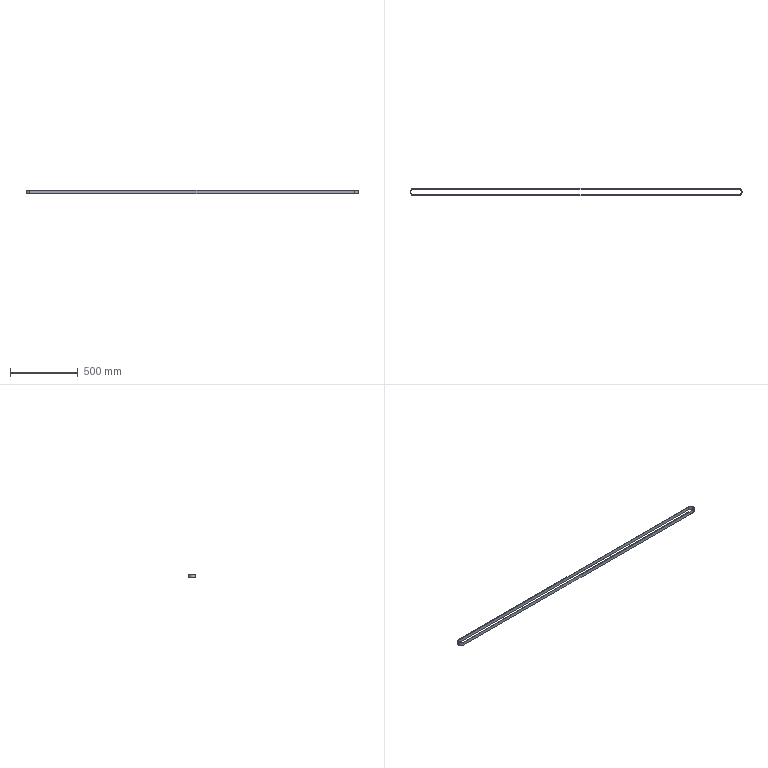Part | STEP file | welding conveyor belt_Default | 1 solid | 12 faces | box 2454 x 51.95 x 25 mm | volume 495464 mm3 | cylinder 6 | plane 6 | commonest cylinder face diameters 43.95 x3 51.95 x3
STEP:
#1=CARTESIAN_POINT('',(0.,0.,0.));
#2=DIRECTION('',(0.,0.,1.));
#3=DIRECTION('',(1.,0.,0.));
#4=AXIS2_PLACEMENT_3D('',#1,#2,#3);
#5=CARTESIAN_POINT('',(2402.,21.975,-25.));
#6=VERTEX_POINT('',#5);
#7=CARTESIAN_POINT('',(2402.,21.975,0.));
#8=VERTEX_POINT('',#7);
#9=CARTESIAN_POINT('',(2402.,21.975,-25.));
#10=DIRECTION('',(0.,0.,1.));
#11=VECTOR('',#10,1.);
#12=LINE('',#9,#11);
#13=CARTESIAN_POINT('',(2402.,0.000000009,-25.));
#14=DIRECTION('',(0.,0.,1.));
#15=DIRECTION('',(1.,0.,0.));
#16=AXIS2_PLACEMENT_3D('',#13,#14,#15);
#17=CYLINDRICAL_SURFACE('',#16,21.975);
#18=CARTESIAN_POINT('',(1.571,0.));
#19=DIRECTION('',(0.,1.));
#20=VECTOR('',#19,1.);
#21=LINE('',#18,#20);
#22=(GEOMETRIC_REPRESENTATION_CONTEXT(2)PARAMETRIC_REPRESENTATION_CONTEXT()REPRESENTATION_CONTEXT('',''));
#23=DEFINITIONAL_REPRESENTATION('',(#21),#22);
#24=PCURVE('',#17,#23);
#25=CARTESIAN_POINT('',(0.,21.975,-25.));
#26=DIRECTION('',(0.,1.,0.));
#27=DIRECTION('',(0.,0.,1.));
#28=AXIS2_PLACEMENT_3D('',#25,#26,#27);
#29=PLANE('',#28);
#30=CARTESIAN_POINT('',(0.,2402.));
#31=DIRECTION('',(1.,0.));
#32=VECTOR('',#31,1.);
#33=LINE('',#30,#32);
#34=(GEOMETRIC_REPRESENTATION_CONTEXT(2)PARAMETRIC_REPRESENTATION_CONTEXT()REPRESENTATION_CONTEXT('',''));
#35=DEFINITIONAL_REPRESENTATION('',(#33),#34);
#36=PCURVE('',#29,#35);
#37=SURFACE_CURVE('',#12,(#24,#36),.PCURVE_S1.);
#38=EDGE_CURVE('',#6,#8,#37,.T.);
#39=ORIENTED_EDGE('',*,*,#38,.T.);
#40=CARTESIAN_POINT('',(2423.975,0.000000009,0.));
#41=VERTEX_POINT('',#40);
#42=CARTESIAN_POINT('',(2402.,0.000000009,0.));
#43=DIRECTION('',(0.,0.,1.));
#44=DIRECTION('',(-1.,0.,0.));
#45=AXIS2_PLACEMENT_3D('',#42,#43,#44);
#46=CIRCLE('',#45,21.975);
#47=CARTESIAN_POINT('',(-3.142,25.));
#48=DIRECTION('',(1.,0.));
#49=VECTOR('',#48,1.);
#50=LINE('',#47,#49);
#51=(GEOMETRIC_REPRESENTATION_CONTEXT(2)PARAMETRIC_REPRESENTATION_CONTEXT()REPRESENTATION_CONTEXT('',''));
#52=DEFINITIONAL_REPRESENTATION('',(#50),#51);
#53=PCURVE('',#17,#52);
#54=CARTESIAN_POINT('',(0.,0.,0.));
#55=DIRECTION('',(0.,0.,-1.));
#56=DIRECTION('',(-1.,0.,0.));
#57=AXIS2_PLACEMENT_3D('',#54,#55,#56);
#58=PLANE('',#57);
#59=CARTESIAN_POINT('',(-2380.025,0.000000009));
#60=CARTESIAN_POINT('',(-2380.025,-38.062));
#61=CARTESIAN_POINT('',(-2412.988,-19.031));
#62=CARTESIAN_POINT('',(-2445.95,0.000000009));
#63=CARTESIAN_POINT('',(-2412.988,19.031));
#64=CARTESIAN_POINT('',(-2380.025,38.062));
#65=CARTESIAN_POINT('',(-2380.025,0.000000009));
#66=(BOUNDED_CURVE()B_SPLINE_CURVE(2,(#59,#60,#61,#62,#63,#64,#65),.UNSPECIFIED.,.T.,.F.)B_SPLINE_CURVE_WITH_KNOTS((1,2,2,2,2,1),(-2.094,0.,2.094,4.189,6.283,8.378),.UNSPECIFIED.)CURVE()GEOMETRIC_REPRESENTATION_ITEM()RATIONAL_B_SPLINE_CURVE((1.,0.5,1.,0.5,1.,0.5,1.))REPRESENTATION_ITEM(''));
#67=(GEOMETRIC_REPRESENTATION_CONTEXT(2)PARAMETRIC_REPRESENTATION_CONTEXT()REPRESENTATION_CONTEXT('',''));
#68=DEFINITIONAL_REPRESENTATION('',(#66),#67);
#69=PCURVE('',#58,#68);
#70=SURFACE_CURVE('',#46,(#53,#69),.PCURVE_S1.);
#71=EDGE_CURVE('',#41,#8,#70,.T.);
#72=ORIENTED_EDGE('',*,*,#71,.F.);
#73=CARTESIAN_POINT('',(2423.975,0.000000009,-25.));
#74=VERTEX_POINT('',#73);
#75=CARTESIAN_POINT('',(2423.975,0.000000009,-25.));
#76=DIRECTION('',(0.,0.,1.));
#77=VECTOR('',#76,1.);
#78=LINE('',#75,#77);
#79=CARTESIAN_POINT('',(0.,0.));
#80=DIRECTION('',(0.,1.));
#81=VECTOR('',#80,1.);
#82=LINE('',#79,#81);
#83=(GEOMETRIC_REPRESENTATION_CONTEXT(2)PARAMETRIC_REPRESENTATION_CONTEXT()REPRESENTATION_CONTEXT('',''));
#84=DEFINITIONAL_REPRESENTATION('',(#82),#83);
#85=PCURVE('',#17,#84);
#86=CARTESIAN_POINT('',(2402.,0.000000009,-25.));
#87=DIRECTION('',(0.,0.,1.));
#88=DIRECTION('',(1.,0.,0.));
#89=AXIS2_PLACEMENT_3D('',#86,#87,#88);
#90=CYLINDRICAL_SURFACE('',#89,21.975);
#91=CARTESIAN_POINT('',(6.283,0.));
#92=DIRECTION('',(0.,1.));
#93=VECTOR('',#92,1.);
#94=LINE('',#91,#93);
#95=(GEOMETRIC_REPRESENTATION_CONTEXT(2)PARAMETRIC_REPRESENTATION_CONTEXT()REPRESENTATION_CONTEXT('',''));
#96=DEFINITIONAL_REPRESENTATION('',(#94),#95);
#97=PCURVE('',#90,#96);
#98=SURFACE_CURVE('',#78,(#85,#97),.PCURVE_S1.);
#99=EDGE_CURVE('',#74,#41,#98,.T.);
#100=ORIENTED_EDGE('',*,*,#99,.F.);
#101=CARTESIAN_POINT('',(2402.,0.000000009,-25.));
#102=DIRECTION('',(0.,0.,1.));
#103=DIRECTION('',(-1.,0.,0.));
#104=AXIS2_PLACEMENT_3D('',#101,#102,#103);
#105=CIRCLE('',#104,21.975);
#106=CARTESIAN_POINT('',(-3.142,0.));
#107=DIRECTION('',(1.,0.));
#108=VECTOR('',#107,1.);
#109=LINE('',#106,#108);
#110=(GEOMETRIC_REPRESENTATION_CONTEXT(2)PARAMETRIC_REPRESENTATION_CONTEXT()REPRESENTATION_CONTEXT('',''));
#111=DEFINITIONAL_REPRESENTATION('',(#109),#110);
#112=PCURVE('',#17,#111);
#113=CARTESIAN_POINT('',(0.,0.,-25.));
#114=DIRECTION('',(0.,0.,-1.));
#115=DIRECTION('',(-1.,0.,0.));
#116=AXIS2_PLACEMENT_3D('',#113,#114,#115);
#117=PLANE('',#116);
#118=CARTESIAN_POINT('',(-2380.025,0.000000009));
#119=CARTESIAN_POINT('',(-2380.025,-38.062));
#120=CARTESIAN_POINT('',(-2412.988,-19.031));
#121=CARTESIAN_POINT('',(-2445.95,0.000000009));
#122=CARTESIAN_POINT('',(-2412.988,19.031));
#123=CARTESIAN_POINT('',(-2380.025,38.062));
#124=CARTESIAN_POINT('',(-2380.025,0.000000009));
#125=(BOUNDED_CURVE()B_SPLINE_CURVE(2,(#118,#119,#120,#121,#122,#123,#124),.UNSPECIFIED.,.T.,.F.)B_SPLINE_CURVE_WITH_KNOTS((1,2,2,2,2,1),(-2.094,0.,2.094,4.189,6.283,8.378),.UNSPECIFIED.)CURVE()GEOMETRIC_REPRESENTATION_ITEM()RATIONAL_B_SPLINE_CURVE((1.,0.5,1.,0.5,1.,0.5,1.))REPRESENTATION_ITEM(''));
#126=(GEOMETRIC_REPRESENTATION_CONTEXT(2)PARAMETRIC_REPRESENTATION_CONTEXT()REPRESENTATION_CONTEXT('',''));
#127=DEFINITIONAL_REPRESENTATION('',(#125),#126);
#128=PCURVE('',#117,#127);
#129=SURFACE_CURVE('',#105,(#112,#128),.PCURVE_S1.);
#130=EDGE_CURVE('',#74,#6,#129,.T.);
#131=ORIENTED_EDGE('',*,*,#130,.T.);
#132=EDGE_LOOP('',(#39,#72,#100,#131));
#133=FACE_BOUND('',#132,.F.);
#134=ADVANCED_FACE('',(#133),#17,.F.);
#135=CARTESIAN_POINT('',(2402.,-25.975,-25.));
#136=VERTEX_POINT('',#135);
#137=CARTESIAN_POINT('',(2427.975,0.000000009,-25.));
#138=VERTEX_POINT('',#137);
#139=CARTESIAN_POINT('',(2402.,0.000000009,-25.));
#140=DIRECTION('',(0.,0.,1.));
#141=DIRECTION('',(-1.,0.,0.));
#142=AXIS2_PLACEMENT_3D('',#139,#140,#141);
#143=CIRCLE('',#142,25.975);
#144=CARTESIAN_POINT('',(2402.,0.000000009,-25.));
#145=DIRECTION('',(0.,0.,1.));
#146=DIRECTION('',(1.,0.,0.));
#147=AXIS2_PLACEMENT_3D('',#144,#145,#146);
#148=CYLINDRICAL_SURFACE('',#147,25.975);
#149=CARTESIAN_POINT('',(3.142,0.));
#150=DIRECTION('',(1.,0.));
#151=VECTOR('',#150,1.);
#152=LINE('',#149,#151);
#153=(GEOMETRIC_REPRESENTATION_CONTEXT(2)PARAMETRIC_REPRESENTATION_CONTEXT()REPRESENTATION_CONTEXT('',''));
#154=DEFINITIONAL_REPRESENTATION('',(#152),#153);
#155=PCURVE('',#148,#154);
#156=CARTESIAN_POINT('',(-2376.025,0.000000009));
#157=CARTESIAN_POINT('',(-2376.025,-44.99));
#158=CARTESIAN_POINT('',(-2414.988,-22.495));
#159=CARTESIAN_POINT('',(-2453.95,0.000000009));
#160=CARTESIAN_POINT('',(-2414.988,22.495));
#161=CARTESIAN_POINT('',(-2376.025,44.99));
#162=CARTESIAN_POINT('',(-2376.025,0.000000009));
#163=(BOUNDED_CURVE()B_SPLINE_CURVE(2,(#156,#157,#158,#159,#160,#161,#162),.UNSPECIFIED.,.T.,.F.)B_SPLINE_CURVE_WITH_KNOTS((1,2,2,2,2,1),(-2.094,0.,2.094,4.189,6.283,8.378),.UNSPECIFIED.)CURVE()GEOMETRIC_REPRESENTATION_ITEM()RATIONAL_B_SPLINE_CURVE((1.,0.5,1.,0.5,1.,0.5,1.))REPRESENTATION_ITEM(''));
#164=(GEOMETRIC_REPRESENTATION_CONTEXT(2)PARAMETRIC_REPRESENTATION_CONTEXT()REPRESENTATION_CONTEXT('',''));
#165=DEFINITIONAL_REPRESENTATION('',(#163),#164);
#166=PCURVE('',#117,#165);
#167=SURFACE_CURVE('',#143,(#155,#166),.PCURVE_S1.);
#168=EDGE_CURVE('',#136,#138,#167,.T.);
#169=ORIENTED_EDGE('',*,*,#168,.T.);
#170=CARTESIAN_POINT('',(2427.975,0.000000009,0.));
#171=VERTEX_POINT('',#170);
#172=CARTESIAN_POINT('',(2427.975,0.000000009,-25.));
#173=DIRECTION('',(0.,0.,1.));
#174=VECTOR('',#173,1.);
#175=LINE('',#172,#174);
#176=CARTESIAN_POINT('',(6.283,0.));
#177=DIRECTION('',(0.,1.));
#178=VECTOR('',#177,1.);
#179=LINE('',#176,#178);
#180=(GEOMETRIC_REPRESENTATION_CONTEXT(2)PARAMETRIC_REPRESENTATION_CONTEXT()REPRESENTATION_CONTEXT('',''));
#181=DEFINITIONAL_REPRESENTATION('',(#179),#180);
#182=PCURVE('',#148,#181);
#183=CARTESIAN_POINT('',(2402.,0.000000009,-25.));
#184=DIRECTION('',(0.,0.,1.));
#185=DIRECTION('',(1.,0.,0.));
#186=AXIS2_PLACEMENT_3D('',#183,#184,#185);
#187=CYLINDRICAL_SURFACE('',#186,25.975);
#188=CARTESIAN_POINT('',(0.,0.));
#189=DIRECTION('',(0.,1.));
#190=VECTOR('',#189,1.);
#191=LINE('',#188,#190);
#192=(GEOMETRIC_REPRESENTATION_CONTEXT(2)PARAMETRIC_REPRESENTATION_CONTEXT()REPRESENTATION_CONTEXT('',''));
#193=DEFINITIONAL_REPRESENTATION('',(#191),#192);
#194=PCURVE('',#187,#193);
#195=SURFACE_CURVE('',#175,(#182,#194),.PCURVE_S1.);
#196=EDGE_CURVE('',#138,#171,#195,.T.);
#197=ORIENTED_EDGE('',*,*,#196,.T.);
#198=CARTESIAN_POINT('',(2402.,-25.975,0.));
#199=VERTEX_POINT('',#198);
#200=CARTESIAN_POINT('',(2402.,0.000000009,0.));
#201=DIRECTION('',(0.,0.,1.));
#202=DIRECTION('',(-1.,0.,0.));
#203=AXIS2_PLACEMENT_3D('',#200,#201,#202);
#204=CIRCLE('',#203,25.975);
#205=CARTESIAN_POINT('',(3.142,25.));
#206=DIRECTION('',(1.,0.));
#207=VECTOR('',#206,1.);
#208=LINE('',#205,#207);
#209=(GEOMETRIC_REPRESENTATION_CONTEXT(2)PARAMETRIC_REPRESENTATION_CONTEXT()REPRESENTATION_CONTEXT('',''));
#210=DEFINITIONAL_REPRESENTATION('',(#208),#209);
#211=PCURVE('',#148,#210);
#212=CARTESIAN_POINT('',(-2376.025,0.000000009));
#213=CARTESIAN_POINT('',(-2376.025,-44.99));
#214=CARTESIAN_POINT('',(-2414.988,-22.495));
#215=CARTESIAN_POINT('',(-2453.95,0.000000009));
#216=CARTESIAN_POINT('',(-2414.988,22.495));
#217=CARTESIAN_POINT('',(-2376.025,44.99));
#218=CARTESIAN_POINT('',(-2376.025,0.000000009));
#219=(BOUNDED_CURVE()B_SPLINE_CURVE(2,(#212,#213,#214,#215,#216,#217,#218),.UNSPECIFIED.,.T.,.F.)B_SPLINE_CURVE_WITH_KNOTS((1,2,2,2,2,1),(-2.094,0.,2.094,4.189,6.283,8.378),.UNSPECIFIED.)CURVE()GEOMETRIC_REPRESENTATION_ITEM()RATIONAL_B_SPLINE_CURVE((1.,0.5,1.,0.5,1.,0.5,1.))REPRESENTATION_ITEM(''));
#220=(GEOMETRIC_REPRESENTATION_CONTEXT(2)PARAMETRIC_REPRESENTATION_CONTEXT()REPRESENTATION_CONTEXT('',''));
#221=DEFINITIONAL_REPRESENTATION('',(#219),#220);
#222=PCURVE('',#58,#221);
#223=SURFACE_CURVE('',#204,(#211,#222),.PCURVE_S1.);
#224=EDGE_CURVE('',#199,#171,#223,.T.);
#225=ORIENTED_EDGE('',*,*,#224,.F.);
#226=CARTESIAN_POINT('',(2402.,-25.975,-25.));
#227=DIRECTION('',(0.,0.,1.));
#228=VECTOR('',#227,1.);
#229=LINE('',#226,#228);
#230=CARTESIAN_POINT('',(4.712,0.));
#231=DIRECTION('',(0.,1.));
#232=VECTOR('',#231,1.);
#233=LINE('',#230,#232);
#234=(GEOMETRIC_REPRESENTATION_CONTEXT(2)PARAMETRIC_REPRESENTATION_CONTEXT()REPRESENTATION_CONTEXT('',''));
#235=DEFINITIONAL_REPRESENTATION('',(#233),#234);
#236=PCURVE('',#148,#235);
#237=CARTESIAN_POINT('',(2402.,-25.975,-25.));
#238=DIRECTION('',(0.,-1.,0.));
#239=DIRECTION('',(1.,0.,0.));
#240=AXIS2_PLACEMENT_3D('',#237,#238,#239);
#241=PLANE('',#240);
#242=CARTESIAN_POINT('',(0.,0.));
#243=DIRECTION('',(0.,1.));
#244=VECTOR('',#243,1.);
#245=LINE('',#242,#244);
#246=(GEOMETRIC_REPRESENTATION_CONTEXT(2)PARAMETRIC_REPRESENTATION_CONTEXT()REPRESENTATION_CONTEXT('',''));
#247=DEFINITIONAL_REPRESENTATION('',(#245),#246);
#248=PCURVE('',#241,#247);
#249=SURFACE_CURVE('',#229,(#236,#248),.PCURVE_S1.);
#250=EDGE_CURVE('',#136,#199,#249,.T.);
#251=ORIENTED_EDGE('',*,*,#250,.F.);
#252=EDGE_LOOP('',(#169,#197,#225,#251));
#253=FACE_BOUND('',#252,.T.);
#254=ADVANCED_FACE('',(#253),#148,.T.);
#255=CARTESIAN_POINT('',(0.,25.975,-25.));
#256=VERTEX_POINT('',#255);
#257=CARTESIAN_POINT('',(0.,-25.975,-25.));
#258=VERTEX_POINT('',#257);
#259=CARTESIAN_POINT('',(0.,0.,-25.));
#260=DIRECTION('',(0.,0.,1.));
#261=DIRECTION('',(-1.,0.,0.));
#262=AXIS2_PLACEMENT_3D('',#259,#260,#261);
#263=CIRCLE('',#262,25.975);
#264=CARTESIAN_POINT('',(25.975,0.));
#265=CARTESIAN_POINT('',(25.975,-44.99));
#266=CARTESIAN_POINT('',(-12.988,-22.495));
#267=CARTESIAN_POINT('',(-51.95,0.));
#268=CARTESIAN_POINT('',(-12.988,22.495));
#269=CARTESIAN_POINT('',(25.975,44.99));
#270=CARTESIAN_POINT('',(25.975,0.));
#271=(BOUNDED_CURVE()B_SPLINE_CURVE(2,(#264,#265,#266,#267,#268,#269,#270),.UNSPECIFIED.,.T.,.F.)B_SPLINE_CURVE_WITH_KNOTS((1,2,2,2,2,1),(-2.094,0.,2.094,4.189,6.283,8.378),.UNSPECIFIED.)CURVE()GEOMETRIC_REPRESENTATION_ITEM()RATIONAL_B_SPLINE_CURVE((1.,0.5,1.,0.5,1.,0.5,1.))REPRESENTATION_ITEM(''));
#272=(GEOMETRIC_REPRESENTATION_CONTEXT(2)PARAMETRIC_REPRESENTATION_CONTEXT()REPRESENTATION_CONTEXT('',''));
#273=DEFINITIONAL_REPRESENTATION('',(#271),#272);
#274=PCURVE('',#117,#273);
#275=CARTESIAN_POINT('',(0.,0.,-25.));
#276=DIRECTION('',(0.,0.,1.));
#277=DIRECTION('',(1.,0.,0.));
#278=AXIS2_PLACEMENT_3D('',#275,#276,#277);
#279=CYLINDRICAL_SURFACE('',#278,25.975);
#280=CARTESIAN_POINT('',(-3.142,0.));
#281=DIRECTION('',(1.,0.));
#282=VECTOR('',#281,1.);
#283=LINE('',#280,#282);
#284=(GEOMETRIC_REPRESENTATION_CONTEXT(2)PARAMETRIC_REPRESENTATION_CONTEXT()REPRESENTATION_CONTEXT('',''));
#285=DEFINITIONAL_REPRESENTATION('',(#283),#284);
#286=PCURVE('',#279,#285);
#287=SURFACE_CURVE('',#263,(#274,#286),.PCURVE_S1.);
#288=EDGE_CURVE('',#256,#258,#287,.T.);
#289=ORIENTED_EDGE('',*,*,#288,.F.);
#290=CARTESIAN_POINT('',(2402.,25.975,-25.));
#291=VERTEX_POINT('',#290);
#292=CARTESIAN_POINT('',(0.,25.975,-25.));
#293=DIRECTION('',(-1.,0.,0.));
#294=VECTOR('',#293,1.);
#295=LINE('',#292,#294);
#296=CARTESIAN_POINT('',(0.,25.975));
#297=DIRECTION('',(1.,0.));
#298=VECTOR('',#297,1.);
#299=LINE('',#296,#298);
#300=(GEOMETRIC_REPRESENTATION_CONTEXT(2)PARAMETRIC_REPRESENTATION_CONTEXT()REPRESENTATION_CONTEXT('',''));
#301=DEFINITIONAL_REPRESENTATION('',(#299),#300);
#302=PCURVE('',#117,#301);
#303=CARTESIAN_POINT('',(0.,25.975,-25.));
#304=DIRECTION('',(0.,1.,0.));
#305=DIRECTION('',(0.,0.,1.));
#306=AXIS2_PLACEMENT_3D('',#303,#304,#305);
#307=PLANE('',#306);
#308=CARTESIAN_POINT('',(0.,0.));
#309=DIRECTION('',(0.,-1.));
#310=VECTOR('',#309,1.);
#311=LINE('',#308,#310);
#312=(GEOMETRIC_REPRESENTATION_CONTEXT(2)PARAMETRIC_REPRESENTATION_CONTEXT()REPRESENTATION_CONTEXT('',''));
#313=DEFINITIONAL_REPRESENTATION('',(#311),#312);
#314=PCURVE('',#307,#313);
#315=SURFACE_CURVE('',#295,(#302,#314),.PCURVE_S1.);
#316=EDGE_CURVE('',#291,#256,#315,.T.);
#317=ORIENTED_EDGE('',*,*,#316,.F.);
#318=CARTESIAN_POINT('',(2402.,0.000000009,-25.));
#319=DIRECTION('',(0.,0.,1.));
#320=DIRECTION('',(-1.,0.,0.));
#321=AXIS2_PLACEMENT_3D('',#318,#319,#320);
#322=CIRCLE('',#321,25.975);
#323=CARTESIAN_POINT('',(-2376.025,0.000000009));
#324=CARTESIAN_POINT('',(-2376.025,-44.99));
#325=CARTESIAN_POINT('',(-2414.988,-22.495));
#326=CARTESIAN_POINT('',(-2453.95,0.000000009));
#327=CARTESIAN_POINT('',(-2414.988,22.495));
#328=CARTESIAN_POINT('',(-2376.025,44.99));
#329=CARTESIAN_POINT('',(-2376.025,0.000000009));
#330=(BOUNDED_CURVE()B_SPLINE_CURVE(2,(#323,#324,#325,#326,#327,#328,#329),.UNSPECIFIED.,.T.,.F.)B_SPLINE_CURVE_WITH_KNOTS((1,2,2,2,2,1),(-2.094,0.,2.094,4.189,6.283,8.378),.UNSPECIFIED.)CURVE()GEOMETRIC_REPRESENTATION_ITEM()RATIONAL_B_SPLINE_CURVE((1.,0.5,1.,0.5,1.,0.5,1.))REPRESENTATION_ITEM(''));
#331=(GEOMETRIC_REPRESENTATION_CONTEXT(2)PARAMETRIC_REPRESENTATION_CONTEXT()REPRESENTATION_CONTEXT('',''));
#332=DEFINITIONAL_REPRESENTATION('',(#330),#331);
#333=PCURVE('',#117,#332);
#334=CARTESIAN_POINT('',(-3.142,0.));
#335=DIRECTION('',(1.,0.));
#336=VECTOR('',#335,1.);
#337=LINE('',#334,#336);
#338=(GEOMETRIC_REPRESENTATION_CONTEXT(2)PARAMETRIC_REPRESENTATION_CONTEXT()REPRESENTATION_CONTEXT('',''));
#339=DEFINITIONAL_REPRESENTATION('',(#337),#338);
#340=PCURVE('',#187,#339);
#341=SURFACE_CURVE('',#322,(#333,#340),.PCURVE_S1.);
#342=EDGE_CURVE('',#138,#291,#341,.T.);
#343=ORIENTED_EDGE('',*,*,#342,.F.);
#344=ORIENTED_EDGE('',*,*,#168,.F.);
#345=CARTESIAN_POINT('',(2402.,-25.975,-25.));
#346=DIRECTION('',(1.,0.,0.));
#347=VECTOR('',#346,1.);
#348=LINE('',#345,#347);
#349=CARTESIAN_POINT('',(-2402.,-25.975));
#350=DIRECTION('',(-1.,0.));
#351=VECTOR('',#350,1.);
#352=LINE('',#349,#351);
#353=(GEOMETRIC_REPRESENTATION_CONTEXT(2)PARAMETRIC_REPRESENTATION_CONTEXT()REPRESENTATION_CONTEXT('',''));
#354=DEFINITIONAL_REPRESENTATION('',(#352),#353);
#355=PCURVE('',#117,#354);
#356=CARTESIAN_POINT('',(0.,0.));
#357=DIRECTION('',(1.,0.));
#358=VECTOR('',#357,1.);
#359=LINE('',#356,#358);
#360=(GEOMETRIC_REPRESENTATION_CONTEXT(2)PARAMETRIC_REPRESENTATION_CONTEXT()REPRESENTATION_CONTEXT('',''));
#361=DEFINITIONAL_REPRESENTATION('',(#359),#360);
#362=PCURVE('',#241,#361);
#363=SURFACE_CURVE('',#348,(#355,#362),.PCURVE_S1.);
#364=EDGE_CURVE('',#258,#136,#363,.T.);
#365=ORIENTED_EDGE('',*,*,#364,.F.);
#366=EDGE_LOOP('',(#289,#317,#343,#344,#365));
#367=FACE_BOUND('',#366,.T.);
#368=CARTESIAN_POINT('',(0.,21.975,-25.));
#369=VERTEX_POINT('',#368);
#370=CARTESIAN_POINT('',(0.,21.975,-25.));
#371=DIRECTION('',(-1.,0.,0.));
#372=VECTOR('',#371,1.);
#373=LINE('',#370,#372);
#374=CARTESIAN_POINT('',(0.,21.975));
#375=DIRECTION('',(1.,0.));
#376=VECTOR('',#375,1.);
#377=LINE('',#374,#376);
#378=(GEOMETRIC_REPRESENTATION_CONTEXT(2)PARAMETRIC_REPRESENTATION_CONTEXT()REPRESENTATION_CONTEXT('',''));
#379=DEFINITIONAL_REPRESENTATION('',(#377),#378);
#380=PCURVE('',#117,#379);
#381=CARTESIAN_POINT('',(0.,0.));
#382=DIRECTION('',(0.,-1.));
#383=VECTOR('',#382,1.);
#384=LINE('',#381,#383);
#385=(GEOMETRIC_REPRESENTATION_CONTEXT(2)PARAMETRIC_REPRESENTATION_CONTEXT()REPRESENTATION_CONTEXT('',''));
#386=DEFINITIONAL_REPRESENTATION('',(#384),#385);
#387=PCURVE('',#29,#386);
#388=SURFACE_CURVE('',#373,(#380,#387),.PCURVE_S1.);
#389=EDGE_CURVE('',#6,#369,#388,.T.);
#390=ORIENTED_EDGE('',*,*,#389,.T.);
#391=CARTESIAN_POINT('',(0.,-21.975,-25.));
#392=VERTEX_POINT('',#391);
#393=CARTESIAN_POINT('',(0.,0.,-25.));
#394=DIRECTION('',(0.,0.,1.));
#395=DIRECTION('',(-1.,0.,0.));
#396=AXIS2_PLACEMENT_3D('',#393,#394,#395);
#397=CIRCLE('',#396,21.975);
#398=CARTESIAN_POINT('',(21.975,0.));
#399=CARTESIAN_POINT('',(21.975,-38.062));
#400=CARTESIAN_POINT('',(-10.988,-19.031));
#401=CARTESIAN_POINT('',(-43.95,0.));
#402=CARTESIAN_POINT('',(-10.988,19.031));
#403=CARTESIAN_POINT('',(21.975,38.062));
#404=CARTESIAN_POINT('',(21.975,0.));
#405=(BOUNDED_CURVE()B_SPLINE_CURVE(2,(#398,#399,#400,#401,#402,#403,#404),.UNSPECIFIED.,.T.,.F.)B_SPLINE_CURVE_WITH_KNOTS((1,2,2,2,2,1),(-2.094,0.,2.094,4.189,6.283,8.378),.UNSPECIFIED.)CURVE()GEOMETRIC_REPRESENTATION_ITEM()RATIONAL_B_SPLINE_CURVE((1.,0.5,1.,0.5,1.,0.5,1.))REPRESENTATION_ITEM(''));
#406=(GEOMETRIC_REPRESENTATION_CONTEXT(2)PARAMETRIC_REPRESENTATION_CONTEXT()REPRESENTATION_CONTEXT('',''));
#407=DEFINITIONAL_REPRESENTATION('',(#405),#406);
#408=PCURVE('',#117,#407);
#409=CARTESIAN_POINT('',(0.,0.,-25.));
#410=DIRECTION('',(0.,0.,1.));
#411=DIRECTION('',(1.,0.,0.));
#412=AXIS2_PLACEMENT_3D('',#409,#410,#411);
#413=CYLINDRICAL_SURFACE('',#412,21.975);
#414=CARTESIAN_POINT('',(-3.142,0.));
#415=DIRECTION('',(1.,0.));
#416=VECTOR('',#415,1.);
#417=LINE('',#414,#416);
#418=(GEOMETRIC_REPRESENTATION_CONTEXT(2)PARAMETRIC_REPRESENTATION_CONTEXT()REPRESENTATION_CONTEXT('',''));
#419=DEFINITIONAL_REPRESENTATION('',(#417),#418);
#420=PCURVE('',#413,#419);
#421=SURFACE_CURVE('',#397,(#408,#420),.PCURVE_S1.);
#422=EDGE_CURVE('',#369,#392,#421,.T.);
#423=ORIENTED_EDGE('',*,*,#422,.T.);
#424=CARTESIAN_POINT('',(2402.,-21.975,-25.));
#425=VERTEX_POINT('',#424);
#426=CARTESIAN_POINT('',(2402.,-21.975,-25.));
#427=DIRECTION('',(1.,0.,0.));
#428=VECTOR('',#427,1.);
#429=LINE('',#426,#428);
#430=CARTESIAN_POINT('',(-2402.,-21.975));
#431=DIRECTION('',(-1.,0.));
#432=VECTOR('',#431,1.);
#433=LINE('',#430,#432);
#434=(GEOMETRIC_REPRESENTATION_CONTEXT(2)PARAMETRIC_REPRESENTATION_CONTEXT()REPRESENTATION_CONTEXT('',''));
#435=DEFINITIONAL_REPRESENTATION('',(#433),#434);
#436=PCURVE('',#117,#435);
#437=CARTESIAN_POINT('',(2402.,-21.975,-25.));
#438=DIRECTION('',(0.,-1.,0.));
#439=DIRECTION('',(1.,0.,0.));
#440=AXIS2_PLACEMENT_3D('',#437,#438,#439);
#441=PLANE('',#440);
#442=CARTESIAN_POINT('',(0.,0.));
#443=DIRECTION('',(1.,0.));
#444=VECTOR('',#443,1.);
#445=LINE('',#442,#444);
#446=(GEOMETRIC_REPRESENTATION_CONTEXT(2)PARAMETRIC_REPRESENTATION_CONTEXT()REPRESENTATION_CONTEXT('',''));
#447=DEFINITIONAL_REPRESENTATION('',(#445),#446);
#448=PCURVE('',#441,#447);
#449=SURFACE_CURVE('',#429,(#436,#448),.PCURVE_S1.);
#450=EDGE_CURVE('',#392,#425,#449,.T.);
#451=ORIENTED_EDGE('',*,*,#450,.T.);
#452=CARTESIAN_POINT('',(2402.,0.000000009,-25.));
#453=DIRECTION('',(0.,0.,1.));
#454=DIRECTION('',(-1.,0.,0.));
#455=AXIS2_PLACEMENT_3D('',#452,#453,#454);
#456=CIRCLE('',#455,21.975);
#457=CARTESIAN_POINT('',(-2380.025,0.000000009));
#458=CARTESIAN_POINT('',(-2380.025,-38.062));
#459=CARTESIAN_POINT('',(-2412.988,-19.031));
#460=CARTESIAN_POINT('',(-2445.95,0.000000009));
#461=CARTESIAN_POINT('',(-2412.988,19.031));
#462=CARTESIAN_POINT('',(-2380.025,38.062));
#463=CARTESIAN_POINT('',(-2380.025,0.000000009));
#464=(BOUNDED_CURVE()B_SPLINE_CURVE(2,(#457,#458,#459,#460,#461,#462,#463),.UNSPECIFIED.,.T.,.F.)B_SPLINE_CURVE_WITH_KNOTS((1,2,2,2,2,1),(-2.094,0.,2.094,4.189,6.283,8.378),.UNSPECIFIED.)CURVE()GEOMETRIC_REPRESENTATION_ITEM()RATIONAL_B_SPLINE_CURVE((1.,0.5,1.,0.5,1.,0.5,1.))REPRESENTATION_ITEM(''));
#465=(GEOMETRIC_REPRESENTATION_CONTEXT(2)PARAMETRIC_REPRESENTATION_CONTEXT()REPRESENTATION_CONTEXT('',''));
#466=DEFINITIONAL_REPRESENTATION('',(#464),#465);
#467=PCURVE('',#117,#466);
#468=CARTESIAN_POINT('',(3.142,0.));
#469=DIRECTION('',(1.,0.));
#470=VECTOR('',#469,1.);
#471=LINE('',#468,#470);
#472=(GEOMETRIC_REPRESENTATION_CONTEXT(2)PARAMETRIC_REPRESENTATION_CONTEXT()REPRESENTATION_CONTEXT('',''));
#473=DEFINITIONAL_REPRESENTATION('',(#471),#472);
#474=PCURVE('',#90,#473);
#475=SURFACE_CURVE('',#456,(#467,#474),.PCURVE_S1.);
#476=EDGE_CURVE('',#425,#74,#475,.T.);
#477=ORIENTED_EDGE('',*,*,#476,.T.);
#478=ORIENTED_EDGE('',*,*,#130,.T.);
#479=EDGE_LOOP('',(#390,#423,#451,#477,#478));
#480=FACE_BOUND('',#479,.T.);
#481=ADVANCED_FACE('',(#367,#480),#117,.T.);
#482=CARTESIAN_POINT('',(0.,25.975,0.));
#483=VERTEX_POINT('',#482);
#484=CARTESIAN_POINT('',(0.,-25.975,0.));
#485=VERTEX_POINT('',#484);
#486=CARTESIAN_POINT('',(0.,0.,0.));
#487=DIRECTION('',(0.,0.,1.));
#488=DIRECTION('',(-1.,0.,0.));
#489=AXIS2_PLACEMENT_3D('',#486,#487,#488);
#490=CIRCLE('',#489,25.975);
#491=CARTESIAN_POINT('',(25.975,0.));
#492=CARTESIAN_POINT('',(25.975,-44.99));
#493=CARTESIAN_POINT('',(-12.988,-22.495));
#494=CARTESIAN_POINT('',(-51.95,0.));
#495=CARTESIAN_POINT('',(-12.988,22.495));
#496=CARTESIAN_POINT('',(25.975,44.99));
#497=CARTESIAN_POINT('',(25.975,0.));
#498=(BOUNDED_CURVE()B_SPLINE_CURVE(2,(#491,#492,#493,#494,#495,#496,#497),.UNSPECIFIED.,.T.,.F.)B_SPLINE_CURVE_WITH_KNOTS((1,2,2,2,2,1),(-2.094,0.,2.094,4.189,6.283,8.378),.UNSPECIFIED.)CURVE()GEOMETRIC_REPRESENTATION_ITEM()RATIONAL_B_SPLINE_CURVE((1.,0.5,1.,0.5,1.,0.5,1.))REPRESENTATION_ITEM(''));
#499=(GEOMETRIC_REPRESENTATION_CONTEXT(2)PARAMETRIC_REPRESENTATION_CONTEXT()REPRESENTATION_CONTEXT('',''));
#500=DEFINITIONAL_REPRESENTATION('',(#498),#499);
#501=PCURVE('',#58,#500);
#502=CARTESIAN_POINT('',(-3.142,25.));
#503=DIRECTION('',(1.,0.));
#504=VECTOR('',#503,1.);
#505=LINE('',#502,#504);
#506=(GEOMETRIC_REPRESENTATION_CONTEXT(2)PARAMETRIC_REPRESENTATION_CONTEXT()REPRESENTATION_CONTEXT('',''));
#507=DEFINITIONAL_REPRESENTATION('',(#505),#506);
#508=PCURVE('',#279,#507);
#509=SURFACE_CURVE('',#490,(#501,#508),.PCURVE_S1.);
#510=EDGE_CURVE('',#483,#485,#509,.T.);
#511=ORIENTED_EDGE('',*,*,#510,.T.);
#512=CARTESIAN_POINT('',(2402.,-25.975,0.));
#513=DIRECTION('',(1.,0.,0.));
#514=VECTOR('',#513,1.);
#515=LINE('',#512,#514);
#516=CARTESIAN_POINT('',(-2402.,-25.975));
#517=DIRECTION('',(-1.,0.));
#518=VECTOR('',#517,1.);
#519=LINE('',#516,#518);
#520=(GEOMETRIC_REPRESENTATION_CONTEXT(2)PARAMETRIC_REPRESENTATION_CONTEXT()REPRESENTATION_CONTEXT('',''));
#521=DEFINITIONAL_REPRESENTATION('',(#519),#520);
#522=PCURVE('',#58,#521);
#523=CARTESIAN_POINT('',(0.,25.));
#524=DIRECTION('',(1.,0.));
#525=VECTOR('',#524,1.);
#526=LINE('',#523,#525);
#527=(GEOMETRIC_REPRESENTATION_CONTEXT(2)PARAMETRIC_REPRESENTATION_CONTEXT()REPRESENTATION_CONTEXT('',''));
#528=DEFINITIONAL_REPRESENTATION('',(#526),#527);
#529=PCURVE('',#241,#528);
#530=SURFACE_CURVE('',#515,(#522,#529),.PCURVE_S1.);
#531=EDGE_CURVE('',#485,#199,#530,.T.);
#532=ORIENTED_EDGE('',*,*,#531,.T.);
#533=ORIENTED_EDGE('',*,*,#224,.T.);
#534=CARTESIAN_POINT('',(2402.,25.975,0.));
#535=VERTEX_POINT('',#534);
#536=CARTESIAN_POINT('',(2402.,0.000000009,0.));
#537=DIRECTION('',(0.,0.,1.));
#538=DIRECTION('',(-1.,0.,0.));
#539=AXIS2_PLACEMENT_3D('',#536,#537,#538);
#540=CIRCLE('',#539,25.975);
#541=CARTESIAN_POINT('',(-2376.025,0.000000009));
#542=CARTESIAN_POINT('',(-2376.025,-44.99));
#543=CARTESIAN_POINT('',(-2414.988,-22.495));
#544=CARTESIAN_POINT('',(-2453.95,0.000000009));
#545=CARTESIAN_POINT('',(-2414.988,22.495));
#546=CARTESIAN_POINT('',(-2376.025,44.99));
#547=CARTESIAN_POINT('',(-2376.025,0.000000009));
#548=(BOUNDED_CURVE()B_SPLINE_CURVE(2,(#541,#542,#543,#544,#545,#546,#547),.UNSPECIFIED.,.T.,.F.)B_SPLINE_CURVE_WITH_KNOTS((1,2,2,2,2,1),(-2.094,0.,2.094,4.189,6.283,8.378),.UNSPECIFIED.)CURVE()GEOMETRIC_REPRESENTATION_ITEM()RATIONAL_B_SPLINE_CURVE((1.,0.5,1.,0.5,1.,0.5,1.))REPRESENTATION_ITEM(''));
#549=(GEOMETRIC_REPRESENTATION_CONTEXT(2)PARAMETRIC_REPRESENTATION_CONTEXT()REPRESENTATION_CONTEXT('',''));
#550=DEFINITIONAL_REPRESENTATION('',(#548),#549);
#551=PCURVE('',#58,#550);
#552=CARTESIAN_POINT('',(-3.142,25.));
#553=DIRECTION('',(1.,0.));
#554=VECTOR('',#553,1.);
#555=LINE('',#552,#554);
#556=(GEOMETRIC_REPRESENTATION_CONTEXT(2)PARAMETRIC_REPRESENTATION_CONTEXT()REPRESENTATION_CONTEXT('',''));
#557=DEFINITIONAL_REPRESENTATION('',(#555),#556);
#558=PCURVE('',#187,#557);
#559=SURFACE_CURVE('',#540,(#551,#558),.PCURVE_S1.);
#560=EDGE_CURVE('',#171,#535,#559,.T.);
#561=ORIENTED_EDGE('',*,*,#560,.T.);
#562=CARTESIAN_POINT('',(0.,25.975,0.));
#563=DIRECTION('',(-1.,0.,0.));
#564=VECTOR('',#563,1.);
#565=LINE('',#562,#564);
#566=CARTESIAN_POINT('',(0.,25.975));
#567=DIRECTION('',(1.,0.));
#568=VECTOR('',#567,1.);
#569=LINE('',#566,#568);
#570=(GEOMETRIC_REPRESENTATION_CONTEXT(2)PARAMETRIC_REPRESENTATION_CONTEXT()REPRESENTATION_CONTEXT('',''));
#571=DEFINITIONAL_REPRESENTATION('',(#569),#570);
#572=PCURVE('',#58,#571);
#573=CARTESIAN_POINT('',(25.,0.));
#574=DIRECTION('',(0.,-1.));
#575=VECTOR('',#574,1.);
#576=LINE('',#573,#575);
#577=(GEOMETRIC_REPRESENTATION_CONTEXT(2)PARAMETRIC_REPRESENTATION_CONTEXT()REPRESENTATION_CONTEXT('',''));
#578=DEFINITIONAL_REPRESENTATION('',(#576),#577);
#579=PCURVE('',#307,#578);
#580=SURFACE_CURVE('',#565,(#572,#579),.PCURVE_S1.);
#581=EDGE_CURVE('',#535,#483,#580,.T.);
#582=ORIENTED_EDGE('',*,*,#581,.T.);
#583=EDGE_LOOP('',(#511,#532,#533,#561,#582));
#584=FACE_BOUND('',#583,.T.);
#585=CARTESIAN_POINT('',(0.,21.975,0.));
#586=VERTEX_POINT('',#585);
#587=CARTESIAN_POINT('',(0.,-21.975,0.));
#588=VERTEX_POINT('',#587);
#589=CARTESIAN_POINT('',(0.,0.,0.));
#590=DIRECTION('',(0.,0.,1.));
#591=DIRECTION('',(-1.,0.,0.));
#592=AXIS2_PLACEMENT_3D('',#589,#590,#591);
#593=CIRCLE('',#592,21.975);
#594=CARTESIAN_POINT('',(21.975,0.));
#595=CARTESIAN_POINT('',(21.975,-38.062));
#596=CARTESIAN_POINT('',(-10.988,-19.031));
#597=CARTESIAN_POINT('',(-43.95,0.));
#598=CARTESIAN_POINT('',(-10.988,19.031));
#599=CARTESIAN_POINT('',(21.975,38.062));
#600=CARTESIAN_POINT('',(21.975,0.));
#601=(BOUNDED_CURVE()B_SPLINE_CURVE(2,(#594,#595,#596,#597,#598,#599,#600),.UNSPECIFIED.,.T.,.F.)B_SPLINE_CURVE_WITH_KNOTS((1,2,2,2,2,1),(-2.094,0.,2.094,4.189,6.283,8.378),.UNSPECIFIED.)CURVE()GEOMETRIC_REPRESENTATION_ITEM()RATIONAL_B_SPLINE_CURVE((1.,0.5,1.,0.5,1.,0.5,1.))REPRESENTATION_ITEM(''));
#602=(GEOMETRIC_REPRESENTATION_CONTEXT(2)PARAMETRIC_REPRESENTATION_CONTEXT()REPRESENTATION_CONTEXT('',''));
#603=DEFINITIONAL_REPRESENTATION('',(#601),#602);
#604=PCURVE('',#58,#603);
#605=CARTESIAN_POINT('',(-3.142,25.));
#606=DIRECTION('',(1.,0.));
#607=VECTOR('',#606,1.);
#608=LINE('',#605,#607);
#609=(GEOMETRIC_REPRESENTATION_CONTEXT(2)PARAMETRIC_REPRESENTATION_CONTEXT()REPRESENTATION_CONTEXT('',''));
#610=DEFINITIONAL_REPRESENTATION('',(#608),#609);
#611=PCURVE('',#413,#610);
#612=SURFACE_CURVE('',#593,(#604,#611),.PCURVE_S1.);
#613=EDGE_CURVE('',#586,#588,#612,.T.);
#614=ORIENTED_EDGE('',*,*,#613,.F.);
#615=CARTESIAN_POINT('',(0.,21.975,0.));
#616=DIRECTION('',(-1.,0.,0.));
#617=VECTOR('',#616,1.);
#618=LINE('',#615,#617);
#619=CARTESIAN_POINT('',(0.,21.975));
#620=DIRECTION('',(1.,0.));
#621=VECTOR('',#620,1.);
#622=LINE('',#619,#621);
#623=(GEOMETRIC_REPRESENTATION_CONTEXT(2)PARAMETRIC_REPRESENTATION_CONTEXT()REPRESENTATION_CONTEXT('',''));
#624=DEFINITIONAL_REPRESENTATION('',(#622),#623);
#625=PCURVE('',#58,#624);
#626=CARTESIAN_POINT('',(25.,0.));
#627=DIRECTION('',(0.,-1.));
#628=VECTOR('',#627,1.);
#629=LINE('',#626,#628);
#630=(GEOMETRIC_REPRESENTATION_CONTEXT(2)PARAMETRIC_REPRESENTATION_CONTEXT()REPRESENTATION_CONTEXT('',''));
#631=DEFINITIONAL_REPRESENTATION('',(#629),#630);
#632=PCURVE('',#29,#631);
#633=SURFACE_CURVE('',#618,(#625,#632),.PCURVE_S1.);
#634=EDGE_CURVE('',#8,#586,#633,.T.);
#635=ORIENTED_EDGE('',*,*,#634,.F.);
#636=ORIENTED_EDGE('',*,*,#71,.F.);
#637=CARTESIAN_POINT('',(2402.,-21.975,0.));
#638=VERTEX_POINT('',#637);
#639=CARTESIAN_POINT('',(2402.,0.000000009,0.));
#640=DIRECTION('',(0.,0.,1.));
#641=DIRECTION('',(-1.,0.,0.));
#642=AXIS2_PLACEMENT_3D('',#639,#640,#641);
#643=CIRCLE('',#642,21.975);
#644=CARTESIAN_POINT('',(-2380.025,0.000000009));
#645=CARTESIAN_POINT('',(-2380.025,-38.062));
#646=CARTESIAN_POINT('',(-2412.988,-19.031));
#647=CARTESIAN_POINT('',(-2445.95,0.000000009));
#648=CARTESIAN_POINT('',(-2412.988,19.031));
#649=CARTESIAN_POINT('',(-2380.025,38.062));
#650=CARTESIAN_POINT('',(-2380.025,0.000000009));
#651=(BOUNDED_CURVE()B_SPLINE_CURVE(2,(#644,#645,#646,#647,#648,#649,#650),.UNSPECIFIED.,.T.,.F.)B_SPLINE_CURVE_WITH_KNOTS((1,2,2,2,2,1),(-2.094,0.,2.094,4.189,6.283,8.378),.UNSPECIFIED.)CURVE()GEOMETRIC_REPRESENTATION_ITEM()RATIONAL_B_SPLINE_CURVE((1.,0.5,1.,0.5,1.,0.5,1.))REPRESENTATION_ITEM(''));
#652=(GEOMETRIC_REPRESENTATION_CONTEXT(2)PARAMETRIC_REPRESENTATION_CONTEXT()REPRESENTATION_CONTEXT('',''));
#653=DEFINITIONAL_REPRESENTATION('',(#651),#652);
#654=PCURVE('',#58,#653);
#655=CARTESIAN_POINT('',(3.142,25.));
#656=DIRECTION('',(1.,0.));
#657=VECTOR('',#656,1.);
#658=LINE('',#655,#657);
#659=(GEOMETRIC_REPRESENTATION_CONTEXT(2)PARAMETRIC_REPRESENTATION_CONTEXT()REPRESENTATION_CONTEXT('',''));
#660=DEFINITIONAL_REPRESENTATION('',(#658),#659);
#661=PCURVE('',#90,#660);
#662=SURFACE_CURVE('',#643,(#654,#661),.PCURVE_S1.);
#663=EDGE_CURVE('',#638,#41,#662,.T.);
#664=ORIENTED_EDGE('',*,*,#663,.F.);
#665=CARTESIAN_POINT('',(2402.,-21.975,0.));
#666=DIRECTION('',(1.,0.,0.));
#667=VECTOR('',#666,1.);
#668=LINE('',#665,#667);
#669=CARTESIAN_POINT('',(-2402.,-21.975));
#670=DIRECTION('',(-1.,0.));
#671=VECTOR('',#670,1.);
#672=LINE('',#669,#671);
#673=(GEOMETRIC_REPRESENTATION_CONTEXT(2)PARAMETRIC_REPRESENTATION_CONTEXT()REPRESENTATION_CONTEXT('',''));
#674=DEFINITIONAL_REPRESENTATION('',(#672),#673);
#675=PCURVE('',#58,#674);
#676=CARTESIAN_POINT('',(0.,25.));
#677=DIRECTION('',(1.,0.));
#678=VECTOR('',#677,1.);
#679=LINE('',#676,#678);
#680=(GEOMETRIC_REPRESENTATION_CONTEXT(2)PARAMETRIC_REPRESENTATION_CONTEXT()REPRESENTATION_CONTEXT('',''));
#681=DEFINITIONAL_REPRESENTATION('',(#679),#680);
#682=PCURVE('',#441,#681);
#683=SURFACE_CURVE('',#668,(#675,#682),.PCURVE_S1.);
#684=EDGE_CURVE('',#588,#638,#683,.T.);
#685=ORIENTED_EDGE('',*,*,#684,.F.);
#686=EDGE_LOOP('',(#614,#635,#636,#664,#685));
#687=FACE_BOUND('',#686,.T.);
#688=ADVANCED_FACE('',(#584,#687),#58,.F.);
#689=ORIENTED_EDGE('',*,*,#510,.F.);
#690=CARTESIAN_POINT('',(0.,25.975,-25.));
#691=DIRECTION('',(0.,0.,1.));
#692=VECTOR('',#691,1.);
#693=LINE('',#690,#692);
#694=CARTESIAN_POINT('',(1.571,0.));
#695=DIRECTION('',(0.,1.));
#696=VECTOR('',#695,1.);
#697=LINE('',#694,#696);
#698=(GEOMETRIC_REPRESENTATION_CONTEXT(2)PARAMETRIC_REPRESENTATION_CONTEXT()REPRESENTATION_CONTEXT('',''));
#699=DEFINITIONAL_REPRESENTATION('',(#697),#698);
#700=PCURVE('',#279,#699);
#701=CARTESIAN_POINT('',(0.,0.));
#702=DIRECTION('',(1.,0.));
#703=VECTOR('',#702,1.);
#704=LINE('',#701,#703);
#705=(GEOMETRIC_REPRESENTATION_CONTEXT(2)PARAMETRIC_REPRESENTATION_CONTEXT()REPRESENTATION_CONTEXT('',''));
#706=DEFINITIONAL_REPRESENTATION('',(#704),#705);
#707=PCURVE('',#307,#706);
#708=SURFACE_CURVE('',#693,(#700,#707),.PCURVE_S1.);
#709=EDGE_CURVE('',#256,#483,#708,.T.);
#710=ORIENTED_EDGE('',*,*,#709,.F.);
#711=ORIENTED_EDGE('',*,*,#288,.T.);
#712=CARTESIAN_POINT('',(0.,-25.975,-25.));
#713=DIRECTION('',(0.,0.,1.));
#714=VECTOR('',#713,1.);
#715=LINE('',#712,#714);
#716=CARTESIAN_POINT('',(4.712,0.));
#717=DIRECTION('',(0.,1.));
#718=VECTOR('',#717,1.);
#719=LINE('',#716,#718);
#720=(GEOMETRIC_REPRESENTATION_CONTEXT(2)PARAMETRIC_REPRESENTATION_CONTEXT()REPRESENTATION_CONTEXT('',''));
#721=DEFINITIONAL_REPRESENTATION('',(#719),#720);
#722=PCURVE('',#279,#721);
#723=CARTESIAN_POINT('',(-2402.,0.));
#724=DIRECTION('',(0.,1.));
#725=VECTOR('',#724,1.);
#726=LINE('',#723,#725);
#727=(GEOMETRIC_REPRESENTATION_CONTEXT(2)PARAMETRIC_REPRESENTATION_CONTEXT()REPRESENTATION_CONTEXT('',''));
#728=DEFINITIONAL_REPRESENTATION('',(#726),#727);
#729=PCURVE('',#241,#728);
#730=SURFACE_CURVE('',#715,(#722,#729),.PCURVE_S1.);
#731=EDGE_CURVE('',#258,#485,#730,.T.);
#732=ORIENTED_EDGE('',*,*,#731,.T.);
#733=EDGE_LOOP('',(#689,#710,#711,#732));
#734=FACE_BOUND('',#733,.T.);
#735=ADVANCED_FACE('',(#734),#279,.T.);
#736=ORIENTED_EDGE('',*,*,#581,.F.);
#737=CARTESIAN_POINT('',(2402.,25.975,-25.));
#738=DIRECTION('',(0.,0.,1.));
#739=VECTOR('',#738,1.);
#740=LINE('',#737,#739);
#741=CARTESIAN_POINT('',(0.,2402.));
#742=DIRECTION('',(1.,0.));
#743=VECTOR('',#742,1.);
#744=LINE('',#741,#743);
#745=(GEOMETRIC_REPRESENTATION_CONTEXT(2)PARAMETRIC_REPRESENTATION_CONTEXT()REPRESENTATION_CONTEXT('',''));
#746=DEFINITIONAL_REPRESENTATION('',(#744),#745);
#747=PCURVE('',#307,#746);
#748=CARTESIAN_POINT('',(1.571,0.));
#749=DIRECTION('',(0.,1.));
#750=VECTOR('',#749,1.);
#751=LINE('',#748,#750);
#752=(GEOMETRIC_REPRESENTATION_CONTEXT(2)PARAMETRIC_REPRESENTATION_CONTEXT()REPRESENTATION_CONTEXT('',''));
#753=DEFINITIONAL_REPRESENTATION('',(#751),#752);
#754=PCURVE('',#187,#753);
#755=SURFACE_CURVE('',#740,(#747,#754),.PCURVE_S1.);
#756=EDGE_CURVE('',#291,#535,#755,.T.);
#757=ORIENTED_EDGE('',*,*,#756,.F.);
#758=ORIENTED_EDGE('',*,*,#316,.T.);
#759=ORIENTED_EDGE('',*,*,#709,.T.);
#760=EDGE_LOOP('',(#736,#757,#758,#759));
#761=FACE_BOUND('',#760,.T.);
#762=ADVANCED_FACE('',(#761),#307,.T.);
#763=ORIENTED_EDGE('',*,*,#196,.F.);
#764=ORIENTED_EDGE('',*,*,#342,.T.);
#765=ORIENTED_EDGE('',*,*,#756,.T.);
#766=ORIENTED_EDGE('',*,*,#560,.F.);
#767=EDGE_LOOP('',(#763,#764,#765,#766));
#768=FACE_BOUND('',#767,.T.);
#769=ADVANCED_FACE('',(#768),#187,.T.);
#770=ORIENTED_EDGE('',*,*,#531,.F.);
#771=ORIENTED_EDGE('',*,*,#731,.F.);
#772=ORIENTED_EDGE('',*,*,#364,.T.);
#773=ORIENTED_EDGE('',*,*,#250,.T.);
#774=EDGE_LOOP('',(#770,#771,#772,#773));
#775=FACE_BOUND('',#774,.T.);
#776=ADVANCED_FACE('',(#775),#241,.T.);
#777=CARTESIAN_POINT('',(0.,21.975,-25.));
#778=DIRECTION('',(0.,0.,1.));
#779=VECTOR('',#778,1.);
#780=LINE('',#777,#779);
#781=CARTESIAN_POINT('',(1.571,0.));
#782=DIRECTION('',(0.,1.));
#783=VECTOR('',#782,1.);
#784=LINE('',#781,#783);
#785=(GEOMETRIC_REPRESENTATION_CONTEXT(2)PARAMETRIC_REPRESENTATION_CONTEXT()REPRESENTATION_CONTEXT('',''));
#786=DEFINITIONAL_REPRESENTATION('',(#784),#785);
#787=PCURVE('',#413,#786);
#788=CARTESIAN_POINT('',(0.,0.));
#789=DIRECTION('',(1.,0.));
#790=VECTOR('',#789,1.);
#791=LINE('',#788,#790);
#792=(GEOMETRIC_REPRESENTATION_CONTEXT(2)PARAMETRIC_REPRESENTATION_CONTEXT()REPRESENTATION_CONTEXT('',''));
#793=DEFINITIONAL_REPRESENTATION('',(#791),#792);
#794=PCURVE('',#29,#793);
#795=SURFACE_CURVE('',#780,(#787,#794),.PCURVE_S1.);
#796=EDGE_CURVE('',#369,#586,#795,.T.);
#797=ORIENTED_EDGE('',*,*,#796,.F.);
#798=ORIENTED_EDGE('',*,*,#422,.T.);
#799=CARTESIAN_POINT('',(0.,-21.975,-25.));
#800=DIRECTION('',(0.,0.,1.));
#801=VECTOR('',#800,1.);
#802=LINE('',#799,#801);
#803=CARTESIAN_POINT('',(4.712,0.));
#804=DIRECTION('',(0.,1.));
#805=VECTOR('',#804,1.);
#806=LINE('',#803,#805);
#807=(GEOMETRIC_REPRESENTATION_CONTEXT(2)PARAMETRIC_REPRESENTATION_CONTEXT()REPRESENTATION_CONTEXT('',''));
#808=DEFINITIONAL_REPRESENTATION('',(#806),#807);
#809=PCURVE('',#413,#808);
#810=CARTESIAN_POINT('',(-2402.,0.));
#811=DIRECTION('',(0.,1.));
#812=VECTOR('',#811,1.);
#813=LINE('',#810,#812);
#814=(GEOMETRIC_REPRESENTATION_CONTEXT(2)PARAMETRIC_REPRESENTATION_CONTEXT()REPRESENTATION_CONTEXT('',''));
#815=DEFINITIONAL_REPRESENTATION('',(#813),#814);
#816=PCURVE('',#441,#815);
#817=SURFACE_CURVE('',#802,(#809,#816),.PCURVE_S1.);
#818=EDGE_CURVE('',#392,#588,#817,.T.);
#819=ORIENTED_EDGE('',*,*,#818,.T.);
#820=ORIENTED_EDGE('',*,*,#613,.F.);
#821=EDGE_LOOP('',(#797,#798,#819,#820));
#822=FACE_BOUND('',#821,.F.);
#823=ADVANCED_FACE('',(#822),#413,.F.);
#824=ORIENTED_EDGE('',*,*,#634,.T.);
#825=ORIENTED_EDGE('',*,*,#796,.F.);
#826=ORIENTED_EDGE('',*,*,#389,.F.);
#827=ORIENTED_EDGE('',*,*,#38,.T.);
#828=EDGE_LOOP('',(#824,#825,#826,#827));
#829=FACE_BOUND('',#828,.T.);
#830=ADVANCED_FACE('',(#829),#29,.F.);
#831=ORIENTED_EDGE('',*,*,#663,.F.);
#832=CARTESIAN_POINT('',(2402.,-21.975,-25.));
#833=DIRECTION('',(0.,0.,1.));
#834=VECTOR('',#833,1.);
#835=LINE('',#832,#834);
#836=CARTESIAN_POINT('',(4.712,0.));
#837=DIRECTION('',(0.,1.));
#838=VECTOR('',#837,1.);
#839=LINE('',#836,#838);
#840=(GEOMETRIC_REPRESENTATION_CONTEXT(2)PARAMETRIC_REPRESENTATION_CONTEXT()REPRESENTATION_CONTEXT('',''));
#841=DEFINITIONAL_REPRESENTATION('',(#839),#840);
#842=PCURVE('',#90,#841);
#843=CARTESIAN_POINT('',(0.,0.));
#844=DIRECTION('',(0.,1.));
#845=VECTOR('',#844,1.);
#846=LINE('',#843,#845);
#847=(GEOMETRIC_REPRESENTATION_CONTEXT(2)PARAMETRIC_REPRESENTATION_CONTEXT()REPRESENTATION_CONTEXT('',''));
#848=DEFINITIONAL_REPRESENTATION('',(#846),#847);
#849=PCURVE('',#441,#848);
#850=SURFACE_CURVE('',#835,(#842,#849),.PCURVE_S1.);
#851=EDGE_CURVE('',#425,#638,#850,.T.);
#852=ORIENTED_EDGE('',*,*,#851,.F.);
#853=ORIENTED_EDGE('',*,*,#476,.T.);
#854=ORIENTED_EDGE('',*,*,#99,.T.);
#855=EDGE_LOOP('',(#831,#852,#853,#854));
#856=FACE_BOUND('',#855,.F.);
#857=ADVANCED_FACE('',(#856),#90,.F.);
#858=ORIENTED_EDGE('',*,*,#684,.T.);
#859=ORIENTED_EDGE('',*,*,#851,.F.);
#860=ORIENTED_EDGE('',*,*,#450,.F.);
#861=ORIENTED_EDGE('',*,*,#818,.T.);
#862=EDGE_LOOP('',(#858,#859,#860,#861));
#863=FACE_BOUND('',#862,.T.);
#864=ADVANCED_FACE('',(#863),#441,.F.);
#865=CLOSED_SHELL('',(#134,#254,#481,#688,#735,#762,#769,#776,#823,#830,#857,#864));
#866=MANIFOLD_SOLID_BREP('',#865);
#867=(LENGTH_UNIT()NAMED_UNIT(*)SI_UNIT(.MILLI.,.METRE.));
#868=UNCERTAINTY_MEASURE_WITH_UNIT(LENGTH_MEASURE(0.0000001),#867,'','');
#869=(NAMED_UNIT(*)PLANE_ANGLE_UNIT()SI_UNIT($,.RADIAN.));
#870=(NAMED_UNIT(*)SI_UNIT($,.STERADIAN.)SOLID_ANGLE_UNIT());
#871=(GEOMETRIC_REPRESENTATION_CONTEXT(3)GLOBAL_UNCERTAINTY_ASSIGNED_CONTEXT((#868))GLOBAL_UNIT_ASSIGNED_CONTEXT((#867,#869,#870))REPRESENTATION_CONTEXT('',''));
#872=ADVANCED_BREP_SHAPE_REPRESENTATION('',(#4,#866),#871);